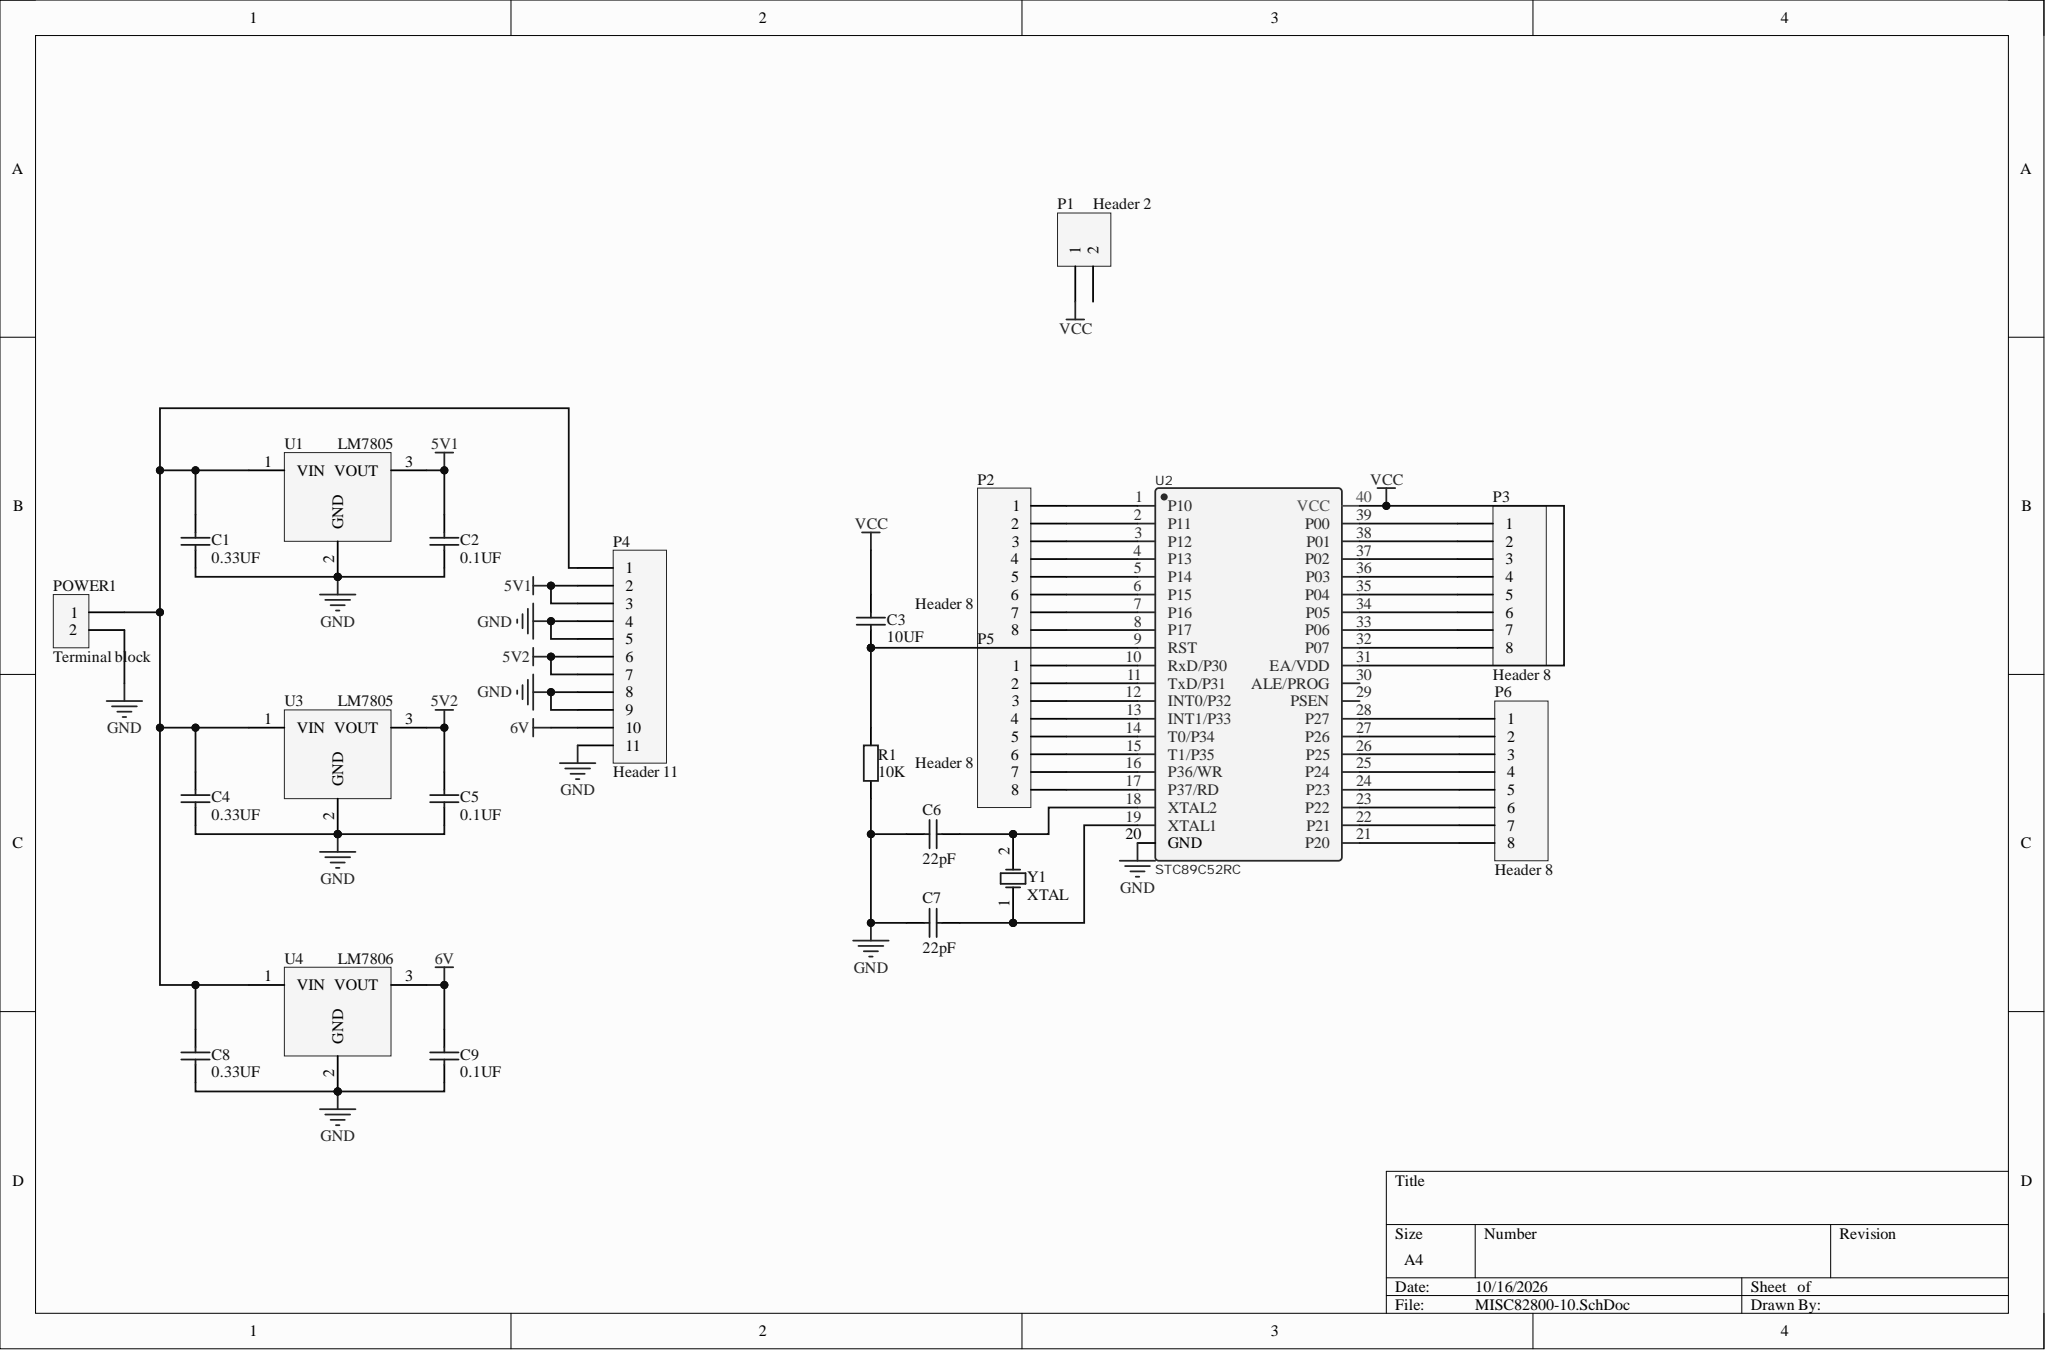Circuit board | Altium Designer | 22 parts | 41 nets
Bill of materials:
Comment,Description,Designator,Footprint,LibRef,Quantity
"0.33UF","Capacitor","C1, C4, C8","RAD-0.3","Cap","3"
"0.1UF","Capacitor","C2, C5, C9","RAD-0.3","Cap","3"
"10UF","Capacitor","C3","RAD-0.3","Cap","1"
"22pF","Capacitor","C6, C7","RAD-0.3","Cap","2"
"Header 2","Header, 2-Pin","P1","HDR1X2","Header 2","1"
"Header 8","Header, 8-Pin","P2, P3, P5, P6","HDR1X8","Header 8","4"
"Header 11","Header, 11-Pin","P4","HDR1X11","Header 11","1"
"Terminal block","","POWER1","VH3.96-2A","VH2","1"
"10K","Resistor","R1","AXIAL-0.4","Res2","1"
"LM7805","","U1, U3","TO220A","LM7805","2"
"STC89C52RC","","U2","STC89C52RC","STC89C52RC","1"
"LM7806","","U4","TO220A","LM7805","1"
"XTAL","Crystal Oscillator","Y1","R38","XTAL","1"
Netlist (Protel format):
[
C1
RAD-0.3
0.33UF



]
[
C2
RAD-0.3
0.1UF



]
[
C3
RAD-0.3
10UF



]
[
C4
RAD-0.3
0.33UF



]
[
C5
RAD-0.3
0.1UF



]
[
C6
RAD-0.3
22pF



]
[
C7
RAD-0.3
22pF



]
[
C8
RAD-0.3
0.33UF



]
[
C9
RAD-0.3
0.1UF



]
[
P1
HDR1X2
Header 2



]
[
P2
HDR1X8
Header 8



]
[
P3
HDR1X8
Header 8



]
[
P4
HDR1X11
Header 11



]
[
P5
HDR1X8
Header 8



]
[
P6
HDR1X8
Header 8



]
[
POWER1
VH3.96-2A
Terminal block



]
[
R1
AXIAL-0.4
10K



]
[
U1
TO220A
LM7805



]
[
U2
STC89C52RC
STC89C52RC



]
[
U3
TO220A
LM7805



]
[
U4
TO220A
LM7806



]
[
Y1
R38
XTAL



]
(
VCC
C3-1
P1-1
U2-31
U2-40
)
(
NetP6_8
P6-8
U2-21
)
(
NetP6_7
P6-7
U2-22
)
(
NetP6_6
P6-6
U2-23
)
(
NetP6_5
P6-5
U2-24
)
(
NetP6_4
P6-4
U2-25
)
(
NetP6_3
P6-3
U2-26
)
(
NetP6_2
P6-2
U2-27
)
(
NetP6_1
P6-1
U2-28
)
(
NetP5_8
P5-8
U2-17
)
(
NetP5_7
P5-7
U2-16
)
(
NetP5_6
P5-6
U2-15
)
(
NetP5_5
P5-5
U2-14
)
(
NetP5_4
P5-4
U2-13
)
(
NetP5_3
P5-3
U2-12
)
(
NetP5_2
P5-2
U2-11
)
(
NetP5_1
P5-1
U2-10
)
(
NetP3_8
P3-8
U2-32
)
(
NetP3_7
P3-7
U2-33
)
(
NetP3_6
P3-6
U2-34
)
(
NetP3_5
P3-5
U2-35
)
(
NetP3_4
P3-4
U2-36
)
(
NetP3_3
P3-3
U2-37
)
(
NetP3_2
P3-2
U2-38
)
(
NetP3_1
P3-1
U2-39
)
(
NetP2_8
P2-8
U2-8
)
(
NetP2_7
P2-7
U2-7
)
(
NetP2_6
P2-6
U2-6
)
(
NetP2_5
P2-5
U2-5
)
(
NetP2_4
P2-4
U2-4
)
(
NetP2_3
P2-3
U2-3
)
(
NetP2_2
P2-2
U2-2
)
(
NetP2_1
P2-1
U2-1
)
(
NetC7_1
C7-1
U2-19
Y1-1
)
(
NetC6_1
C6-1
U2-18
Y1-2
)
(
NetC3_2
C3-2
R1-2
U2-9
)
(
NetC1_1
C1-1
C4-1
C8-1
P4-1
POWER1-1
U1-1
U3-1
U4-1
)
(
GND
C1-2
C2-2
C4-2
C5-2
C6-2
C7-2
C8-2
C9-2
P4-4
P4-5
P4-8
P4-9
P4-11
POWER1-2
R1-1
U1-2
U2-20
U3-2
U4-2
)
(
6V
C9-1
P4-10
U4-3
)
(
5V2
C5-1
P4-6
P4-7
U3-3
)
(
5V1
C2-1
P4-2
P4-3
U1-3
)